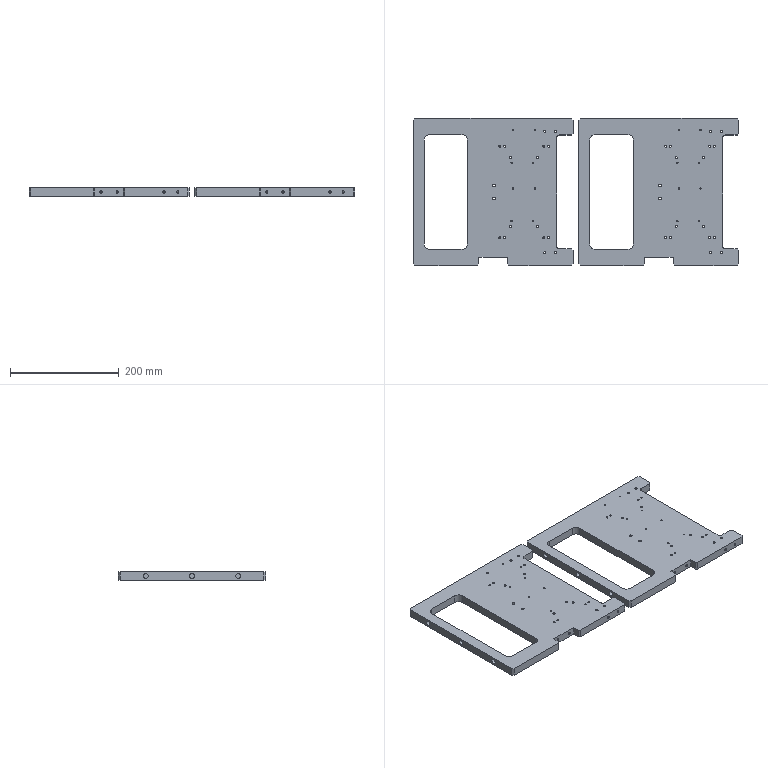CAM job | NX | 3-axis milling, drilling | part box 600 x 271 x 15 mm | stock box 605 x 276 x 15 mm
Tools:
number,name,description,diameter,corner_radius,flute_length,length,flutes
9,D10,平底铣刀-粗,10.0,0.0,35.0,75.0,2
11,D2-J,平底铣刀-精,2.0,0.0,50.0,75.0,2
18,D3-J,平底铣刀-精,3.0,0.0,50.0,75.0,2
7,D6-J,平底铣刀-精,6.0,0.0,25.0,75.0,2
2,D6倒角刀,倒角刀,6.0,0.0,3.0,25.0,2
12,ZT2.6,钻头,2.6,0.0,35.0,50.0,2
13,ZT3.4,钻头,3.4,0.0,35.0,50.0,2
15,ZT5.1,钻头,5.1,0.0,35.0,50.0,2
17,ZT3.9,Drilling Tool,3.9,0.0,35.0,50.0,2
14,ZT4.3,Drilling Tool,4.3,0.0,50.0,75.0,4
Operations:
program,operation,operation_type,tool,method,geometry_group,spindle_rpm,surface_speed,feed_per_tooth,feed_cut,feed_plunge,cut_length_mm,path_length_mm,cut_time_min,machine_time_min
B,C0.3封闭铣廓倒角6X45L_COPY,PlanarMilling,D6倒角刀,爬面_倒角-切深0-步距G,W-B,7000.0,131.0,0.1071,1500.0,100.0,573.667,669.667,0.3824,0.392
B,C0.3封闭铣廓倒角6X45L_COPY_1,PlanarMilling,D6倒角刀,爬面_倒角-切深0-步距G,W-B,7000.0,131.0,0.1071,1500.0,100.0,1219.473,1315.473,0.813,0.8226
B,钻倒角_5,Operation,D6倒角刀,METHOD,W-B,8000.0,150.796,0.0625,1000.0,0.0,38.0,526.397,0.038,0.0868
B,钻倒角_6,Operation,D6倒角刀,METHOD,W-B,8000.0,150.796,0.0625,1000.0,0.0,41.6,554.299,0.0416,0.0929
B,钻倒角_7,Operation,D6倒角刀,METHOD,W-B,8000.0,150.796,0.0625,1000.0,0.0,21.2,378.615,0.0212,0.0569
B,钻倒角_8,Operation,D6倒角刀,METHOD,W-B,8000.0,150.796,0.0625,1000.0,0.0,22.8,419.068,0.0228,0.0624
B,C0.3封闭铣廓倒角6X45L_COPY_2,PlanarMilling,D6倒角刀,爬面_倒角-切深0-步距G,W-B,7000.0,131.0,0.1071,1500.0,100.0,49.086,266.06,0.0327,0.0544
B,铣倒角_2,PlanarMilling,D6倒角刀,METHOD,W-B,8000.0,150.796,0.0375,600.0,100.0,37.911,267.25,0.0632,0.0861
A,打点,Operation,D6倒角刀,METHOD,W-A,3000.0,56.549,0.0333,200.0,0.0,32.0,1062.065,0.16,0.263
A,打点_2,Operation,D6倒角刀,METHOD,W-A,3000.0,56.549,0.0333,200.0,0.0,90.0,1517.888,0.45,0.5928
A,打孔,Operation,ZT2.6,METHOD,W-A,3800.0,29.845,0.0105,80.0,0.0,248.0,1494.065,3.1,3.225
A,打孔_2,Operation,ZT3.4,METHOD,W-A,3500.0,36.285,0.0143,100.0,0.0,248.0,1482.979,2.48,2.603
A,打孔_3,Operation,ZT3.9,METHOD,W-A,3000.0,35.814,0.02,120.0,0.0,124.0,1024.55,1.033,1.123
A,打孔_4,Operation,ZT4.3,METHOD,W-A,3000.0,39.584,0.0167,100.0,0.0,124.0,1128.606,1.24,1.341
A,打孔_5,Operation,ZT5.1,METHOD,W-A,2800.0,43.982,0.0214,120.0,0.0,62.0,540.543,0.5167,0.5645
A,框开粗_1,VolumeBased25DMillingOperation,D10,METHOD,W-A,6000.0,188.0,0.25,4000.0,80.0,33035.846,33557.146,8.259,8.311
A,外形粗_2,VolumeBased25DMillingOperation,D10,METHOD,W-A,6000.0,188.0,0.25,4000.0,80.0,76277.242,76728.497,19.069,19.114
A,框半精_1,VolumeBased25DMillingOperation,D6-J,METHOD,W-A,6000.0,113.0,0.0833,1000.0,100.0,2204.431,2803.681,2.204,2.264
A,框精_1,VolumeBased25DMillingOperation,D6-J,METHOD,W-A,6000.0,113.0,0.0833,1000.0,100.0,1101.816,1701.605,1.102,1.162
A,底壁铣螺旋精光-中_COPY,VolumeBased25DMillingOperation,D2-J,螺旋精光-切深K-步距G,W-A,8000.0,50.266,0.0312,500.0,100.0,2218.158,4296.998,4.436,4.644
A,等高光顺清角D2参考6_COPY,ZLevelMilling,D2-J,分层精光-切深K-步距G,W-A,8000.0,50.266,0.125,2000.0,100.0,3997.036,4526.738,1.998,2.051
A,底壁铣螺旋精光-中_COPY_COPY_1,VolumeBased25DMillingOperation,D3-J,螺旋精光-切深K-步距G,W-A,8000.0,50.266,0.0312,500.0,100.0,1857.74,3714.215,3.716,3.901
A,仅选体,SurfaceContour,D6倒角刀,METHOD,W-A,6000.0,113.0,0.125,1200.0,100.0,3569.264,4465.85,2.974,3.064
A,钻倒角_1,Operation,D6倒角刀,METHOD,W-A,5000.0,94.248,0.015,150.0,0.0,76.0,1181.311,0.5067,0.6172
A,钻倒角_2,Operation,D6倒角刀,METHOD,W-A,5000.0,94.248,0.015,150.0,0.0,83.2,1187.119,0.5547,0.6651
A,钻倒角_3,Operation,D6倒角刀,METHOD,W-A,5000.0,94.248,0.015,150.0,0.0,42.4,875.748,0.2827,0.366
A,钻倒角_4,Operation,D6倒角刀,METHOD,W-A,5000.0,94.248,0.015,150.0,0.0,45.6,986.651,0.304,0.3981
A,铣倒角_1,PlanarMilling,D6倒角刀,METHOD,W-A,6000.0,113.097,0.05,600.0,100.0,70.289,672.591,0.1171,0.1774
A,底壁铣螺旋精光-中_COPY_COPY,VolumeBased25DMillingOperation,D2-J,螺旋精光-切深K-步距G,W-A,8000.0,50.266,0.0187,300.0,100.0,1667.496,2963.516,5.558,5.688
A,外形半精_2,VolumeBased25DMillingOperation,D6-J,METHOD,W-A,6000.0,113.0,0.0833,1000.0,100.0,4895.336,5527.729,4.895,4.959
A,外形精_2,VolumeBased25DMillingOperation,D6-J,METHOD,W-A,6000.0,113.0,0.0833,1000.0,100.0,2447.279,2927.475,2.447,2.495